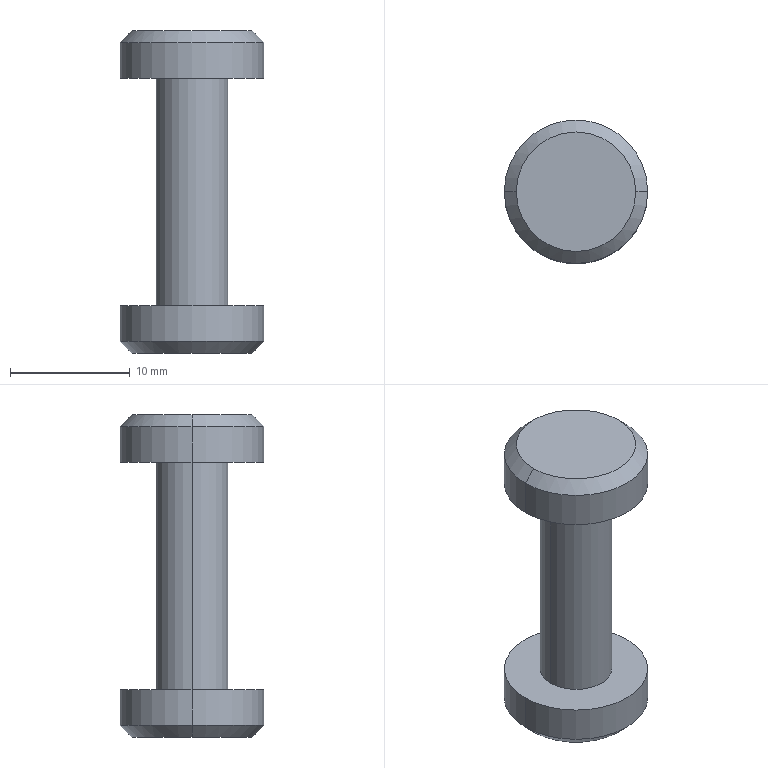Part | SolidWorks | features Chamfer 2, ICE 2, Extrusion 1 | 1 solid | 14 faces | box 12 x 12 x 27 mm | volume 1406 mm3 | cylinder 6 | cone 4 | plane 4 | commonest cylinder face diameters 12 x4 6 x2
STEP:
#1=CARTESIAN_POINT('',(-5.,0.,-4.));
#2=VERTEX_POINT('',#1);
#3=CARTESIAN_POINT('',(5.,0.,-4.));
#4=VERTEX_POINT('',#3);
#5=CARTESIAN_POINT('',(0.,0.,-4.));
#6=DIRECTION('',(0.,0.,-1.));
#7=DIRECTION('',(-1.,0.,0.));
#8=AXIS2_PLACEMENT_3D('',#5,#6,#7);
#9=CIRCLE('',#8,5.);
#10=EDGE_CURVE('',#2,#4,#9,.T.);
#11=ORIENTED_EDGE('',*,*,#10,.F.);
#12=CARTESIAN_POINT('',(-6.,0.,-3.));
#13=VERTEX_POINT('',#12);
#14=CARTESIAN_POINT('',(-5.,0.,-4.));
#15=DIRECTION('',(-0.7071,0.,0.7071));
#16=VECTOR('',#15,1000.);
#17=LINE('',#14,#16);
#18=EDGE_CURVE('',#2,#13,#17,.T.);
#19=ORIENTED_EDGE('',*,*,#18,.T.);
#20=CARTESIAN_POINT('',(6.,0.,-3.));
#21=VERTEX_POINT('',#20);
#22=CARTESIAN_POINT('',(0.,0.,-3.));
#23=DIRECTION('',(0.,0.,1.));
#24=DIRECTION('',(-1.,0.,0.));
#25=AXIS2_PLACEMENT_3D('',#22,#23,#24);
#26=CIRCLE('',#25,6.);
#27=EDGE_CURVE('',#21,#13,#26,.T.);
#28=ORIENTED_EDGE('',*,*,#27,.F.);
#29=CARTESIAN_POINT('',(5.,0.,-4.));
#30=DIRECTION('',(0.7071,0.,0.7071));
#31=VECTOR('',#30,1000.);
#32=LINE('',#29,#31);
#33=EDGE_CURVE('',#4,#21,#32,.T.);
#34=ORIENTED_EDGE('',*,*,#33,.F.);
#35=EDGE_LOOP('',(#11,#19,#28,#34));
#36=FACE_OUTER_BOUND('',#35,.T.);
#37=CARTESIAN_POINT('',(0.,0.,-4.));
#38=DIRECTION('',(0.,0.,1.));
#39=DIRECTION('',(1.,0.,0.));
#40=AXIS2_PLACEMENT_3D('',#37,#38,#39);
#41=CONICAL_SURFACE('',#40,5.,0.7854);
#42=ADVANCED_FACE('',(#36),#41,.T.);
#43=ORIENTED_EDGE('',*,*,#27,.T.);
#44=CARTESIAN_POINT('',(-6.,0.,0.));
#45=VERTEX_POINT('',#44);
#46=CARTESIAN_POINT('',(-6.,0.,-4.));
#47=DIRECTION('',(0.,0.,1.));
#48=VECTOR('',#47,1000.);
#49=LINE('',#46,#48);
#50=EDGE_CURVE('',#13,#45,#49,.T.);
#51=ORIENTED_EDGE('',*,*,#50,.T.);
#52=CARTESIAN_POINT('',(6.,0.,0.));
#53=VERTEX_POINT('',#52);
#54=CARTESIAN_POINT('',(0.,0.,0.));
#55=DIRECTION('',(0.,0.,-1.));
#56=DIRECTION('',(-1.,0.,0.));
#57=AXIS2_PLACEMENT_3D('',#54,#55,#56);
#58=CIRCLE('',#57,6.);
#59=EDGE_CURVE('',#45,#53,#58,.T.);
#60=ORIENTED_EDGE('',*,*,#59,.T.);
#61=CARTESIAN_POINT('',(6.,0.,-4.));
#62=DIRECTION('',(0.,0.,1.));
#63=VECTOR('',#62,1000.);
#64=LINE('',#61,#63);
#65=EDGE_CURVE('',#21,#53,#64,.T.);
#66=ORIENTED_EDGE('',*,*,#65,.F.);
#67=EDGE_LOOP('',(#43,#51,#60,#66));
#68=FACE_OUTER_BOUND('',#67,.T.);
#69=CARTESIAN_POINT('',(0.,0.,-4.));
#70=DIRECTION('',(0.,0.,1.));
#71=DIRECTION('',(1.,0.,0.));
#72=AXIS2_PLACEMENT_3D('',#69,#70,#71);
#73=CYLINDRICAL_SURFACE('',#72,6.);
#74=ADVANCED_FACE('',(#68),#73,.T.);
#75=CARTESIAN_POINT('',(5.,0.,23.));
#76=VERTEX_POINT('',#75);
#77=CARTESIAN_POINT('',(-5.,0.,23.));
#78=VERTEX_POINT('',#77);
#79=CARTESIAN_POINT('',(0.,0.,23.));
#80=DIRECTION('',(0.,0.,1.));
#81=DIRECTION('',(1.,0.,0.));
#82=AXIS2_PLACEMENT_3D('',#79,#80,#81);
#83=CIRCLE('',#82,5.);
#84=EDGE_CURVE('',#76,#78,#83,.T.);
#85=ORIENTED_EDGE('',*,*,#84,.F.);
#86=CARTESIAN_POINT('',(6.,0.,22.));
#87=VERTEX_POINT('',#86);
#88=CARTESIAN_POINT('',(5.,0.,23.));
#89=DIRECTION('',(0.7071,0.,-0.7071));
#90=VECTOR('',#89,1000.);
#91=LINE('',#88,#90);
#92=EDGE_CURVE('',#76,#87,#91,.T.);
#93=ORIENTED_EDGE('',*,*,#92,.T.);
#94=CARTESIAN_POINT('',(-6.,0.,22.));
#95=VERTEX_POINT('',#94);
#96=CARTESIAN_POINT('',(0.,0.,22.));
#97=DIRECTION('',(0.,0.,-1.));
#98=DIRECTION('',(1.,0.,0.));
#99=AXIS2_PLACEMENT_3D('',#96,#97,#98);
#100=CIRCLE('',#99,6.);
#101=EDGE_CURVE('',#95,#87,#100,.T.);
#102=ORIENTED_EDGE('',*,*,#101,.F.);
#103=CARTESIAN_POINT('',(-5.,0.,23.));
#104=DIRECTION('',(-0.7071,0.,-0.7071));
#105=VECTOR('',#104,1000.);
#106=LINE('',#103,#105);
#107=EDGE_CURVE('',#78,#95,#106,.T.);
#108=ORIENTED_EDGE('',*,*,#107,.F.);
#109=EDGE_LOOP('',(#85,#93,#102,#108));
#110=FACE_OUTER_BOUND('',#109,.T.);
#111=CARTESIAN_POINT('',(0.,0.,23.));
#112=DIRECTION('',(0.,0.,-1.));
#113=DIRECTION('',(-1.,0.,0.));
#114=AXIS2_PLACEMENT_3D('',#111,#112,#113);
#115=CONICAL_SURFACE('',#114,5.,0.7854);
#116=ADVANCED_FACE('',(#110),#115,.T.);
#117=ORIENTED_EDGE('',*,*,#101,.T.);
#118=CARTESIAN_POINT('',(6.,0.,19.));
#119=VERTEX_POINT('',#118);
#120=CARTESIAN_POINT('',(6.,0.,23.));
#121=DIRECTION('',(0.,0.,-1.));
#122=VECTOR('',#121,1000.);
#123=LINE('',#120,#122);
#124=EDGE_CURVE('',#87,#119,#123,.T.);
#125=ORIENTED_EDGE('',*,*,#124,.T.);
#126=CARTESIAN_POINT('',(-6.,0.,19.));
#127=VERTEX_POINT('',#126);
#128=CARTESIAN_POINT('',(0.,0.,19.));
#129=DIRECTION('',(0.,0.,1.));
#130=DIRECTION('',(1.,0.,0.));
#131=AXIS2_PLACEMENT_3D('',#128,#129,#130);
#132=CIRCLE('',#131,6.);
#133=EDGE_CURVE('',#119,#127,#132,.T.);
#134=ORIENTED_EDGE('',*,*,#133,.T.);
#135=CARTESIAN_POINT('',(-6.,0.,23.));
#136=DIRECTION('',(0.,0.,-1.));
#137=VECTOR('',#136,1000.);
#138=LINE('',#135,#137);
#139=EDGE_CURVE('',#95,#127,#138,.T.);
#140=ORIENTED_EDGE('',*,*,#139,.F.);
#141=EDGE_LOOP('',(#117,#125,#134,#140));
#142=FACE_OUTER_BOUND('',#141,.T.);
#143=CARTESIAN_POINT('',(0.,0.,23.));
#144=DIRECTION('',(0.,0.,-1.));
#145=DIRECTION('',(-1.,0.,0.));
#146=AXIS2_PLACEMENT_3D('',#143,#144,#145);
#147=CYLINDRICAL_SURFACE('',#146,6.);
#148=ADVANCED_FACE('',(#142),#147,.T.);
#149=CARTESIAN_POINT('',(3.,0.,19.));
#150=VERTEX_POINT('',#149);
#151=CARTESIAN_POINT('',(-3.,0.,19.));
#152=VERTEX_POINT('',#151);
#153=CARTESIAN_POINT('',(0.,0.,19.));
#154=DIRECTION('',(0.,0.,1.));
#155=DIRECTION('',(1.,0.,0.));
#156=AXIS2_PLACEMENT_3D('',#153,#154,#155);
#157=CIRCLE('',#156,3.);
#158=EDGE_CURVE('',#150,#152,#157,.T.);
#159=ORIENTED_EDGE('',*,*,#158,.F.);
#160=CARTESIAN_POINT('',(3.,0.,0.));
#161=VERTEX_POINT('',#160);
#162=CARTESIAN_POINT('',(3.,0.,19.));
#163=DIRECTION('',(0.,0.,-1.));
#164=VECTOR('',#163,1000.);
#165=LINE('',#162,#164);
#166=EDGE_CURVE('',#150,#161,#165,.T.);
#167=ORIENTED_EDGE('',*,*,#166,.T.);
#168=CARTESIAN_POINT('',(-3.,0.,0.));
#169=VERTEX_POINT('',#168);
#170=CARTESIAN_POINT('',(0.,0.,0.));
#171=DIRECTION('',(0.,0.,1.));
#172=DIRECTION('',(1.,0.,0.));
#173=AXIS2_PLACEMENT_3D('',#170,#171,#172);
#174=CIRCLE('',#173,3.);
#175=EDGE_CURVE('',#161,#169,#174,.T.);
#176=ORIENTED_EDGE('',*,*,#175,.T.);
#177=CARTESIAN_POINT('',(-3.,0.,19.));
#178=DIRECTION('',(0.,0.,-1.));
#179=VECTOR('',#178,1000.);
#180=LINE('',#177,#179);
#181=EDGE_CURVE('',#152,#169,#180,.T.);
#182=ORIENTED_EDGE('',*,*,#181,.F.);
#183=EDGE_LOOP('',(#159,#167,#176,#182));
#184=FACE_OUTER_BOUND('',#183,.T.);
#185=CARTESIAN_POINT('',(0.,0.,19.));
#186=DIRECTION('',(0.,0.,-1.));
#187=DIRECTION('',(-1.,0.,0.));
#188=AXIS2_PLACEMENT_3D('',#185,#186,#187);
#189=CYLINDRICAL_SURFACE('',#188,3.);
#190=ADVANCED_FACE('',(#184),#189,.T.);
#191=ORIENTED_EDGE('',*,*,#166,.F.);
#192=CARTESIAN_POINT('',(0.,0.,19.));
#193=DIRECTION('',(0.,0.,1.));
#194=DIRECTION('',(1.,0.,0.));
#195=AXIS2_PLACEMENT_3D('',#192,#193,#194);
#196=CIRCLE('',#195,3.);
#197=EDGE_CURVE('',#152,#150,#196,.T.);
#198=ORIENTED_EDGE('',*,*,#197,.F.);
#199=ORIENTED_EDGE('',*,*,#181,.T.);
#200=CARTESIAN_POINT('',(0.,0.,0.));
#201=DIRECTION('',(0.,0.,1.));
#202=DIRECTION('',(1.,0.,0.));
#203=AXIS2_PLACEMENT_3D('',#200,#201,#202);
#204=CIRCLE('',#203,3.);
#205=EDGE_CURVE('',#169,#161,#204,.T.);
#206=ORIENTED_EDGE('',*,*,#205,.T.);
#207=EDGE_LOOP('',(#191,#198,#199,#206));
#208=FACE_OUTER_BOUND('',#207,.T.);
#209=CARTESIAN_POINT('',(0.,0.,19.));
#210=DIRECTION('',(0.,0.,-1.));
#211=DIRECTION('',(-1.,0.,0.));
#212=AXIS2_PLACEMENT_3D('',#209,#210,#211);
#213=CYLINDRICAL_SURFACE('',#212,3.);
#214=ADVANCED_FACE('',(#208),#213,.T.);
#215=ORIENTED_EDGE('',*,*,#124,.F.);
#216=CARTESIAN_POINT('',(0.,0.,22.));
#217=DIRECTION('',(0.,0.,-1.));
#218=DIRECTION('',(1.,0.,0.));
#219=AXIS2_PLACEMENT_3D('',#216,#217,#218);
#220=CIRCLE('',#219,6.);
#221=EDGE_CURVE('',#87,#95,#220,.T.);
#222=ORIENTED_EDGE('',*,*,#221,.T.);
#223=ORIENTED_EDGE('',*,*,#139,.T.);
#224=CARTESIAN_POINT('',(0.,0.,19.));
#225=DIRECTION('',(0.,0.,1.));
#226=DIRECTION('',(1.,0.,0.));
#227=AXIS2_PLACEMENT_3D('',#224,#225,#226);
#228=CIRCLE('',#227,6.);
#229=EDGE_CURVE('',#127,#119,#228,.T.);
#230=ORIENTED_EDGE('',*,*,#229,.T.);
#231=EDGE_LOOP('',(#215,#222,#223,#230));
#232=FACE_OUTER_BOUND('',#231,.T.);
#233=CARTESIAN_POINT('',(0.,0.,23.));
#234=DIRECTION('',(0.,0.,-1.));
#235=DIRECTION('',(-1.,0.,0.));
#236=AXIS2_PLACEMENT_3D('',#233,#234,#235);
#237=CYLINDRICAL_SURFACE('',#236,6.);
#238=ADVANCED_FACE('',(#232),#237,.T.);
#239=CARTESIAN_POINT('',(0.,0.,23.));
#240=DIRECTION('',(0.,0.,1.));
#241=DIRECTION('',(1.,0.,0.));
#242=AXIS2_PLACEMENT_3D('',#239,#240,#241);
#243=CIRCLE('',#242,5.);
#244=EDGE_CURVE('',#78,#76,#243,.T.);
#245=ORIENTED_EDGE('',*,*,#244,.T.);
#246=ORIENTED_EDGE('',*,*,#84,.T.);
#247=EDGE_LOOP('',(#245,#246));
#248=FACE_OUTER_BOUND('',#247,.T.);
#249=CARTESIAN_POINT('',(0.,0.,23.));
#250=DIRECTION('',(0.,0.,1.));
#251=DIRECTION('',(1.,0.,0.));
#252=AXIS2_PLACEMENT_3D('',#249,#250,#251);
#253=PLANE('',#252);
#254=ADVANCED_FACE('',(#248),#253,.T.);
#255=ORIENTED_EDGE('',*,*,#197,.T.);
#256=ORIENTED_EDGE('',*,*,#158,.T.);
#257=EDGE_LOOP('',(#255,#256));
#258=FACE_BOUND('',#257,.T.);
#259=ORIENTED_EDGE('',*,*,#229,.F.);
#260=ORIENTED_EDGE('',*,*,#133,.F.);
#261=EDGE_LOOP('',(#259,#260));
#262=FACE_OUTER_BOUND('',#261,.T.);
#263=CARTESIAN_POINT('',(0.,0.,19.));
#264=DIRECTION('',(0.,0.,1.));
#265=DIRECTION('',(1.,0.,0.));
#266=AXIS2_PLACEMENT_3D('',#263,#264,#265);
#267=PLANE('',#266);
#268=ADVANCED_FACE('',(#258,#262),#267,.F.);
#269=ORIENTED_EDGE('',*,*,#92,.F.);
#270=ORIENTED_EDGE('',*,*,#244,.F.);
#271=ORIENTED_EDGE('',*,*,#107,.T.);
#272=ORIENTED_EDGE('',*,*,#221,.F.);
#273=EDGE_LOOP('',(#269,#270,#271,#272));
#274=FACE_OUTER_BOUND('',#273,.T.);
#275=CARTESIAN_POINT('',(0.,0.,23.));
#276=DIRECTION('',(0.,0.,-1.));
#277=DIRECTION('',(-1.,0.,0.));
#278=AXIS2_PLACEMENT_3D('',#275,#276,#277);
#279=CONICAL_SURFACE('',#278,5.,0.7854);
#280=ADVANCED_FACE('',(#274),#279,.T.);
#281=ORIENTED_EDGE('',*,*,#50,.F.);
#282=CARTESIAN_POINT('',(0.,0.,-3.));
#283=DIRECTION('',(0.,0.,1.));
#284=DIRECTION('',(-1.,0.,0.));
#285=AXIS2_PLACEMENT_3D('',#282,#283,#284);
#286=CIRCLE('',#285,6.);
#287=EDGE_CURVE('',#13,#21,#286,.T.);
#288=ORIENTED_EDGE('',*,*,#287,.T.);
#289=ORIENTED_EDGE('',*,*,#65,.T.);
#290=CARTESIAN_POINT('',(0.,0.,0.));
#291=DIRECTION('',(0.,0.,-1.));
#292=DIRECTION('',(-1.,0.,0.));
#293=AXIS2_PLACEMENT_3D('',#290,#291,#292);
#294=CIRCLE('',#293,6.);
#295=EDGE_CURVE('',#53,#45,#294,.T.);
#296=ORIENTED_EDGE('',*,*,#295,.T.);
#297=EDGE_LOOP('',(#281,#288,#289,#296));
#298=FACE_OUTER_BOUND('',#297,.T.);
#299=CARTESIAN_POINT('',(0.,0.,-4.));
#300=DIRECTION('',(0.,0.,1.));
#301=DIRECTION('',(1.,0.,0.));
#302=AXIS2_PLACEMENT_3D('',#299,#300,#301);
#303=CYLINDRICAL_SURFACE('',#302,6.);
#304=ADVANCED_FACE('',(#298),#303,.T.);
#305=CARTESIAN_POINT('',(0.,0.,-4.));
#306=DIRECTION('',(0.,0.,-1.));
#307=DIRECTION('',(-1.,0.,0.));
#308=AXIS2_PLACEMENT_3D('',#305,#306,#307);
#309=CIRCLE('',#308,5.);
#310=EDGE_CURVE('',#4,#2,#309,.T.);
#311=ORIENTED_EDGE('',*,*,#310,.T.);
#312=ORIENTED_EDGE('',*,*,#10,.T.);
#313=EDGE_LOOP('',(#311,#312));
#314=FACE_OUTER_BOUND('',#313,.T.);
#315=CARTESIAN_POINT('',(0.,0.,-4.));
#316=DIRECTION('',(0.,0.,-1.));
#317=DIRECTION('',(-1.,0.,0.));
#318=AXIS2_PLACEMENT_3D('',#315,#316,#317);
#319=PLANE('',#318);
#320=ADVANCED_FACE('',(#314),#319,.T.);
#321=ORIENTED_EDGE('',*,*,#205,.F.);
#322=ORIENTED_EDGE('',*,*,#175,.F.);
#323=EDGE_LOOP('',(#321,#322));
#324=FACE_BOUND('',#323,.T.);
#325=ORIENTED_EDGE('',*,*,#295,.F.);
#326=ORIENTED_EDGE('',*,*,#59,.F.);
#327=EDGE_LOOP('',(#325,#326));
#328=FACE_OUTER_BOUND('',#327,.T.);
#329=CARTESIAN_POINT('',(0.,0.,0.));
#330=DIRECTION('',(0.,0.,-1.));
#331=DIRECTION('',(-1.,0.,0.));
#332=AXIS2_PLACEMENT_3D('',#329,#330,#331);
#333=PLANE('',#332);
#334=ADVANCED_FACE('',(#324,#328),#333,.F.);
#335=ORIENTED_EDGE('',*,*,#18,.F.);
#336=ORIENTED_EDGE('',*,*,#310,.F.);
#337=ORIENTED_EDGE('',*,*,#33,.T.);
#338=ORIENTED_EDGE('',*,*,#287,.F.);
#339=EDGE_LOOP('',(#335,#336,#337,#338));
#340=FACE_OUTER_BOUND('',#339,.T.);
#341=CARTESIAN_POINT('',(0.,0.,-4.));
#342=DIRECTION('',(0.,0.,1.));
#343=DIRECTION('',(1.,0.,0.));
#344=AXIS2_PLACEMENT_3D('',#341,#342,#343);
#345=CONICAL_SURFACE('',#344,5.,0.7854);
#346=ADVANCED_FACE('',(#340),#345,.T.);
#347=CLOSED_SHELL('',(#42,#74,#116,#148,#190,#214,#238,#254,#268,#280,#304,#320,#334,#346));
#348=MANIFOLD_SOLID_BREP('',#347);
#349=CARTESIAN_POINT('',(0.,0.,0.));
#350=DIRECTION('',(0.,0.,1.));
#351=DIRECTION('',(1.,0.,0.));
#352=AXIS2_PLACEMENT_3D('',#349,#350,#351);
#353=(LENGTH_UNIT()NAMED_UNIT(*)SI_UNIT(.MILLI.,.METRE.));
#354=UNCERTAINTY_MEASURE_WITH_UNIT(LENGTH_MEASURE(0.00001),#353,'','');
#355=(NAMED_UNIT(*)PLANE_ANGLE_UNIT()SI_UNIT($,.RADIAN.));
#356=(NAMED_UNIT(*)SI_UNIT($,.STERADIAN.)SOLID_ANGLE_UNIT());
#357=(GEOMETRIC_REPRESENTATION_CONTEXT(3)GLOBAL_UNCERTAINTY_ASSIGNED_CONTEXT((#354))GLOBAL_UNIT_ASSIGNED_CONTEXT((#353,#355,#356))REPRESENTATION_CONTEXT('',''));
#358=ADVANCED_BREP_SHAPE_REPRESENTATION('',(#348,#352),#357);